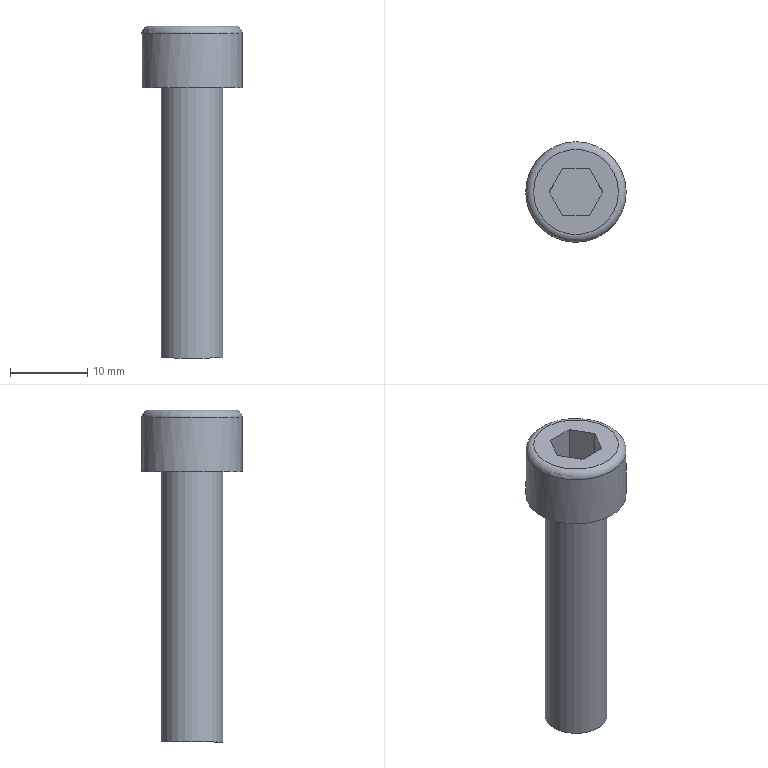Part | STEP file | Tube necking machine_id262_x_t | 1 solid | 13 faces | box 13 x 13 x 43 mm | volume 2648 mm3 | plane 10 | cylinder 2 | torus 1 | commonest cylinder face diameters 8 x1 13 x1
STEP:
#1=CARTESIAN_POINT('',(0.,0.,0.));
#2=DIRECTION('',(0.,0.,1.));
#3=DIRECTION('',(1.,0.,0.));
#4=AXIS2_PLACEMENT_3D('',#1,#2,#3);
#5=CARTESIAN_POINT('',(42.5,122.,246.));
#6=VERTEX_POINT('',#5);
#7=CARTESIAN_POINT('',(48.,122.,246.));
#8=DIRECTION('',(0.,0.,1.));
#9=DIRECTION('',(-1.,0.,0.));
#10=AXIS2_PLACEMENT_3D('',#7,#8,#9);
#11=CIRCLE('',#10,5.5);
#12=CARTESIAN_POINT('',(54.5,122.,246.));
#13=DIRECTION('',(0.,0.,-1.));
#14=DIRECTION('',(-1.,0.,0.));
#15=AXIS2_PLACEMENT_3D('',#12,#13,#14);
#16=PLANE('',#15);
#17=CARTESIAN_POINT('',(12.,0.));
#18=CARTESIAN_POINT('',(12.,-9.526));
#19=CARTESIAN_POINT('',(3.75,-4.763));
#20=CARTESIAN_POINT('',(-4.5,0.));
#21=CARTESIAN_POINT('',(3.75,4.763));
#22=CARTESIAN_POINT('',(12.,9.526));
#23=CARTESIAN_POINT('',(12.,0.));
#24=(BOUNDED_CURVE()B_SPLINE_CURVE(2,(#17,#18,#19,#20,#21,#22,#23),.UNSPECIFIED.,.T.,.F.)B_SPLINE_CURVE_WITH_KNOTS((1,2,2,2,2,1),(-2.094,0.,2.094,4.189,6.283,8.378),.UNSPECIFIED.)CURVE()GEOMETRIC_REPRESENTATION_ITEM()RATIONAL_B_SPLINE_CURVE((1.,0.5,1.,0.5,1.,0.5,1.))REPRESENTATION_ITEM(''));
#25=(GEOMETRIC_REPRESENTATION_CONTEXT(2)PARAMETRIC_REPRESENTATION_CONTEXT()REPRESENTATION_CONTEXT('',''));
#26=DEFINITIONAL_REPRESENTATION('',(#24),#25);
#27=PCURVE('',#16,#26);
#28=CARTESIAN_POINT('',(48.,122.,245.));
#29=DIRECTION('',(0.,0.,-1.));
#30=DIRECTION('',(-1.,0.,0.));
#31=AXIS2_PLACEMENT_3D('',#28,#29,#30);
#32=TOROIDAL_SURFACE('',#31,5.5,1.);
#33=CARTESIAN_POINT('',(6.283,4.712));
#34=DIRECTION('',(-1.,0.));
#35=VECTOR('',#34,1.);
#36=LINE('',#33,#35);
#37=(GEOMETRIC_REPRESENTATION_CONTEXT(2)PARAMETRIC_REPRESENTATION_CONTEXT()REPRESENTATION_CONTEXT('',''));
#38=DEFINITIONAL_REPRESENTATION('',(#36),#37);
#39=PCURVE('',#32,#38);
#40=SURFACE_CURVE('',#11,(#27,#39),.PCURVE_S1.);
#41=EDGE_CURVE('',#6,#6,#40,.T.);
#42=ORIENTED_EDGE('',*,*,#41,.T.);
#43=EDGE_LOOP('',(#42));
#44=FACE_BOUND('',#43,.T.);
#45=CARTESIAN_POINT('',(49.732,119.,246.));
#46=VERTEX_POINT('',#45);
#47=CARTESIAN_POINT('',(46.268,119.,246.));
#48=VERTEX_POINT('',#47);
#49=CARTESIAN_POINT('',(46.268,119.,246.));
#50=DIRECTION('',(-1.,0.,0.));
#51=VECTOR('',#50,1.);
#52=LINE('',#49,#51);
#53=CARTESIAN_POINT('',(8.232,-3.));
#54=DIRECTION('',(1.,0.));
#55=VECTOR('',#54,1.);
#56=LINE('',#53,#55);
#57=(GEOMETRIC_REPRESENTATION_CONTEXT(2)PARAMETRIC_REPRESENTATION_CONTEXT()REPRESENTATION_CONTEXT('',''));
#58=DEFINITIONAL_REPRESENTATION('',(#56),#57);
#59=PCURVE('',#16,#58);
#60=CARTESIAN_POINT('',(46.268,119.,240.72));
#61=DIRECTION('',(0.,1.,0.));
#62=DIRECTION('',(1.,0.,0.));
#63=AXIS2_PLACEMENT_3D('',#60,#61,#62);
#64=PLANE('',#63);
#65=CARTESIAN_POINT('',(0.,-5.28));
#66=DIRECTION('',(-1.,0.));
#67=VECTOR('',#66,1.);
#68=LINE('',#65,#67);
#69=(GEOMETRIC_REPRESENTATION_CONTEXT(2)PARAMETRIC_REPRESENTATION_CONTEXT()REPRESENTATION_CONTEXT('',''));
#70=DEFINITIONAL_REPRESENTATION('',(#68),#69);
#71=PCURVE('',#64,#70);
#72=SURFACE_CURVE('',#52,(#59,#71),.PCURVE_S1.);
#73=EDGE_CURVE('',#46,#48,#72,.T.);
#74=ORIENTED_EDGE('',*,*,#73,.T.);
#75=CARTESIAN_POINT('',(44.536,122.,246.));
#76=VERTEX_POINT('',#75);
#77=CARTESIAN_POINT('',(44.536,122.,246.));
#78=DIRECTION('',(-0.5,0.866,0.));
#79=VECTOR('',#78,1.);
#80=LINE('',#77,#79);
#81=CARTESIAN_POINT('',(9.964,0.));
#82=DIRECTION('',(0.5,0.866));
#83=VECTOR('',#82,1.);
#84=LINE('',#81,#83);
#85=(GEOMETRIC_REPRESENTATION_CONTEXT(2)PARAMETRIC_REPRESENTATION_CONTEXT()REPRESENTATION_CONTEXT('',''));
#86=DEFINITIONAL_REPRESENTATION('',(#84),#85);
#87=PCURVE('',#16,#86);
#88=CARTESIAN_POINT('',(44.536,122.,240.72));
#89=DIRECTION('',(0.866,0.5,0.));
#90=DIRECTION('',(0.5,-0.866,0.));
#91=AXIS2_PLACEMENT_3D('',#88,#89,#90);
#92=PLANE('',#91);
#93=CARTESIAN_POINT('',(0.,-5.28));
#94=DIRECTION('',(-1.,0.));
#95=VECTOR('',#94,1.);
#96=LINE('',#93,#95);
#97=(GEOMETRIC_REPRESENTATION_CONTEXT(2)PARAMETRIC_REPRESENTATION_CONTEXT()REPRESENTATION_CONTEXT('',''));
#98=DEFINITIONAL_REPRESENTATION('',(#96),#97);
#99=PCURVE('',#92,#98);
#100=SURFACE_CURVE('',#80,(#87,#99),.PCURVE_S1.);
#101=EDGE_CURVE('',#48,#76,#100,.T.);
#102=ORIENTED_EDGE('',*,*,#101,.T.);
#103=CARTESIAN_POINT('',(46.268,125.,246.));
#104=VERTEX_POINT('',#103);
#105=CARTESIAN_POINT('',(46.268,125.,246.));
#106=DIRECTION('',(0.5,0.866,0.));
#107=VECTOR('',#106,1.);
#108=LINE('',#105,#107);
#109=CARTESIAN_POINT('',(8.232,3.));
#110=DIRECTION('',(-0.5,0.866));
#111=VECTOR('',#110,1.);
#112=LINE('',#109,#111);
#113=(GEOMETRIC_REPRESENTATION_CONTEXT(2)PARAMETRIC_REPRESENTATION_CONTEXT()REPRESENTATION_CONTEXT('',''));
#114=DEFINITIONAL_REPRESENTATION('',(#112),#113);
#115=PCURVE('',#16,#114);
#116=CARTESIAN_POINT('',(46.268,125.,240.72));
#117=DIRECTION('',(0.866,-0.5,0.));
#118=DIRECTION('',(-0.5,-0.866,0.));
#119=AXIS2_PLACEMENT_3D('',#116,#117,#118);
#120=PLANE('',#119);
#121=CARTESIAN_POINT('',(0.,-5.28));
#122=DIRECTION('',(-1.,0.));
#123=VECTOR('',#122,1.);
#124=LINE('',#121,#123);
#125=(GEOMETRIC_REPRESENTATION_CONTEXT(2)PARAMETRIC_REPRESENTATION_CONTEXT()REPRESENTATION_CONTEXT('',''));
#126=DEFINITIONAL_REPRESENTATION('',(#124),#125);
#127=PCURVE('',#120,#126);
#128=SURFACE_CURVE('',#108,(#115,#127),.PCURVE_S1.);
#129=EDGE_CURVE('',#76,#104,#128,.T.);
#130=ORIENTED_EDGE('',*,*,#129,.T.);
#131=CARTESIAN_POINT('',(49.732,125.,246.));
#132=VERTEX_POINT('',#131);
#133=CARTESIAN_POINT('',(49.732,125.,246.));
#134=DIRECTION('',(1.,0.,0.));
#135=VECTOR('',#134,1.);
#136=LINE('',#133,#135);
#137=CARTESIAN_POINT('',(4.768,3.));
#138=DIRECTION('',(-1.,0.));
#139=VECTOR('',#138,1.);
#140=LINE('',#137,#139);
#141=(GEOMETRIC_REPRESENTATION_CONTEXT(2)PARAMETRIC_REPRESENTATION_CONTEXT()REPRESENTATION_CONTEXT('',''));
#142=DEFINITIONAL_REPRESENTATION('',(#140),#141);
#143=PCURVE('',#16,#142);
#144=CARTESIAN_POINT('',(49.732,125.,240.72));
#145=DIRECTION('',(0.,-1.,0.));
#146=DIRECTION('',(-1.,0.,0.));
#147=AXIS2_PLACEMENT_3D('',#144,#145,#146);
#148=PLANE('',#147);
#149=CARTESIAN_POINT('',(0.,-5.28));
#150=DIRECTION('',(-1.,0.));
#151=VECTOR('',#150,1.);
#152=LINE('',#149,#151);
#153=(GEOMETRIC_REPRESENTATION_CONTEXT(2)PARAMETRIC_REPRESENTATION_CONTEXT()REPRESENTATION_CONTEXT('',''));
#154=DEFINITIONAL_REPRESENTATION('',(#152),#153);
#155=PCURVE('',#148,#154);
#156=SURFACE_CURVE('',#136,(#143,#155),.PCURVE_S1.);
#157=EDGE_CURVE('',#104,#132,#156,.T.);
#158=ORIENTED_EDGE('',*,*,#157,.T.);
#159=CARTESIAN_POINT('',(51.464,122.,246.));
#160=VERTEX_POINT('',#159);
#161=CARTESIAN_POINT('',(51.464,122.,246.));
#162=DIRECTION('',(0.5,-0.866,0.));
#163=VECTOR('',#162,1.);
#164=LINE('',#161,#163);
#165=CARTESIAN_POINT('',(3.036,0.));
#166=DIRECTION('',(-0.5,-0.866));
#167=VECTOR('',#166,1.);
#168=LINE('',#165,#167);
#169=(GEOMETRIC_REPRESENTATION_CONTEXT(2)PARAMETRIC_REPRESENTATION_CONTEXT()REPRESENTATION_CONTEXT('',''));
#170=DEFINITIONAL_REPRESENTATION('',(#168),#169);
#171=PCURVE('',#16,#170);
#172=CARTESIAN_POINT('',(51.464,122.,240.72));
#173=DIRECTION('',(-0.866,-0.5,0.));
#174=DIRECTION('',(-0.5,0.866,0.));
#175=AXIS2_PLACEMENT_3D('',#172,#173,#174);
#176=PLANE('',#175);
#177=CARTESIAN_POINT('',(0.,-5.28));
#178=DIRECTION('',(-1.,0.));
#179=VECTOR('',#178,1.);
#180=LINE('',#177,#179);
#181=(GEOMETRIC_REPRESENTATION_CONTEXT(2)PARAMETRIC_REPRESENTATION_CONTEXT()REPRESENTATION_CONTEXT('',''));
#182=DEFINITIONAL_REPRESENTATION('',(#180),#181);
#183=PCURVE('',#176,#182);
#184=SURFACE_CURVE('',#164,(#171,#183),.PCURVE_S1.);
#185=EDGE_CURVE('',#132,#160,#184,.T.);
#186=ORIENTED_EDGE('',*,*,#185,.T.);
#187=CARTESIAN_POINT('',(49.732,119.,246.));
#188=DIRECTION('',(-0.5,-0.866,0.));
#189=VECTOR('',#188,1.);
#190=LINE('',#187,#189);
#191=CARTESIAN_POINT('',(4.768,-3.));
#192=DIRECTION('',(0.5,-0.866));
#193=VECTOR('',#192,1.);
#194=LINE('',#191,#193);
#195=(GEOMETRIC_REPRESENTATION_CONTEXT(2)PARAMETRIC_REPRESENTATION_CONTEXT()REPRESENTATION_CONTEXT('',''));
#196=DEFINITIONAL_REPRESENTATION('',(#194),#195);
#197=PCURVE('',#16,#196);
#198=CARTESIAN_POINT('',(49.732,119.,240.72));
#199=DIRECTION('',(-0.866,0.5,0.));
#200=DIRECTION('',(0.5,0.866,0.));
#201=AXIS2_PLACEMENT_3D('',#198,#199,#200);
#202=PLANE('',#201);
#203=CARTESIAN_POINT('',(0.,-5.28));
#204=DIRECTION('',(-1.,0.));
#205=VECTOR('',#204,1.);
#206=LINE('',#203,#205);
#207=(GEOMETRIC_REPRESENTATION_CONTEXT(2)PARAMETRIC_REPRESENTATION_CONTEXT()REPRESENTATION_CONTEXT('',''));
#208=DEFINITIONAL_REPRESENTATION('',(#206),#207);
#209=PCURVE('',#202,#208);
#210=SURFACE_CURVE('',#190,(#197,#209),.PCURVE_S1.);
#211=EDGE_CURVE('',#160,#46,#210,.T.);
#212=ORIENTED_EDGE('',*,*,#211,.T.);
#213=EDGE_LOOP('',(#74,#102,#130,#158,#186,#212));
#214=FACE_BOUND('',#213,.T.);
#215=ADVANCED_FACE('',(#44,#214),#16,.F.);
#216=CARTESIAN_POINT('',(41.5,122.,245.));
#217=VERTEX_POINT('',#216);
#218=CARTESIAN_POINT('',(54.5,122.,245.));
#219=VERTEX_POINT('',#218);
#220=CARTESIAN_POINT('',(48.,122.,245.));
#221=DIRECTION('',(0.,0.,-1.));
#222=DIRECTION('',(-1.,0.,0.));
#223=AXIS2_PLACEMENT_3D('',#220,#221,#222);
#224=CIRCLE('',#223,6.5);
#225=CARTESIAN_POINT('',(48.,122.,216.1));
#226=DIRECTION('',(0.,0.,1.));
#227=DIRECTION('',(1.,0.,0.));
#228=AXIS2_PLACEMENT_3D('',#225,#226,#227);
#229=CYLINDRICAL_SURFACE('',#228,6.5);
#230=CARTESIAN_POINT('',(3.142,28.9));
#231=DIRECTION('',(-1.,0.));
#232=VECTOR('',#231,1.);
#233=LINE('',#230,#232);
#234=(GEOMETRIC_REPRESENTATION_CONTEXT(2)PARAMETRIC_REPRESENTATION_CONTEXT()REPRESENTATION_CONTEXT('',''));
#235=DEFINITIONAL_REPRESENTATION('',(#233),#234);
#236=PCURVE('',#229,#235);
#237=CARTESIAN_POINT('',(0.,6.283));
#238=DIRECTION('',(1.,0.));
#239=VECTOR('',#238,1.);
#240=LINE('',#237,#239);
#241=(GEOMETRIC_REPRESENTATION_CONTEXT(2)PARAMETRIC_REPRESENTATION_CONTEXT()REPRESENTATION_CONTEXT('',''));
#242=DEFINITIONAL_REPRESENTATION('',(#240),#241);
#243=PCURVE('',#32,#242);
#244=SURFACE_CURVE('',#224,(#236,#243),.PCURVE_S1.);
#245=EDGE_CURVE('',#217,#219,#244,.T.);
#246=ORIENTED_EDGE('',*,*,#245,.T.);
#247=CARTESIAN_POINT('',(54.5,122.,238.));
#248=VERTEX_POINT('',#247);
#249=CARTESIAN_POINT('',(54.5,122.,238.));
#250=CARTESIAN_POINT('',(54.5,122.,245.));
#251=B_SPLINE_CURVE_WITH_KNOTS('',1,(#249,#250),.UNSPECIFIED.,.F.,.F.,(2,2),(21.9,28.9),.PIECEWISE_BEZIER_KNOTS.);
#252=CARTESIAN_POINT('',(0.,0.));
#253=DIRECTION('',(0.,1.));
#254=VECTOR('',#253,1.);
#255=LINE('',#252,#254);
#256=(GEOMETRIC_REPRESENTATION_CONTEXT(2)PARAMETRIC_REPRESENTATION_CONTEXT()REPRESENTATION_CONTEXT('',''));
#257=DEFINITIONAL_REPRESENTATION('',(#255),#256);
#258=PCURVE('',#229,#257);
#259=CARTESIAN_POINT('',(6.283,0.));
#260=DIRECTION('',(0.,1.));
#261=VECTOR('',#260,1.);
#262=LINE('',#259,#261);
#263=(GEOMETRIC_REPRESENTATION_CONTEXT(2)PARAMETRIC_REPRESENTATION_CONTEXT()REPRESENTATION_CONTEXT('',''));
#264=DEFINITIONAL_REPRESENTATION('',(#262),#263);
#265=PCURVE('',#229,#264);
#266=SEAM_CURVE('',#251,(#258,#265),.PCURVE_S1.);
#267=EDGE_CURVE('',#248,#219,#266,.T.);
#268=ORIENTED_EDGE('',*,*,#267,.F.);
#269=CARTESIAN_POINT('',(48.,122.,238.));
#270=DIRECTION('',(0.,0.,1.));
#271=DIRECTION('',(1.,0.,0.));
#272=AXIS2_PLACEMENT_3D('',#269,#270,#271);
#273=CIRCLE('',#272,6.5);
#274=CARTESIAN_POINT('',(0.,21.9));
#275=DIRECTION('',(1.,0.));
#276=VECTOR('',#275,1.);
#277=LINE('',#274,#276);
#278=(GEOMETRIC_REPRESENTATION_CONTEXT(2)PARAMETRIC_REPRESENTATION_CONTEXT()REPRESENTATION_CONTEXT('',''));
#279=DEFINITIONAL_REPRESENTATION('',(#277),#278);
#280=PCURVE('',#229,#279);
#281=CARTESIAN_POINT('',(52.,122.,238.));
#282=DIRECTION('',(0.,0.,1.));
#283=DIRECTION('',(1.,0.,0.));
#284=AXIS2_PLACEMENT_3D('',#281,#282,#283);
#285=PLANE('',#284);
#286=CARTESIAN_POINT('',(-4.,0.));
#287=DIRECTION('',(1.,0.));
#288=AXIS2_PLACEMENT_2D('',#286,#287);
#289=CIRCLE('',#288,6.5);
#290=(GEOMETRIC_REPRESENTATION_CONTEXT(2)PARAMETRIC_REPRESENTATION_CONTEXT()REPRESENTATION_CONTEXT('',''));
#291=DEFINITIONAL_REPRESENTATION('',(#289),#290);
#292=PCURVE('',#285,#291);
#293=SURFACE_CURVE('',#273,(#280,#292),.PCURVE_S1.);
#294=EDGE_CURVE('',#248,#248,#293,.T.);
#295=ORIENTED_EDGE('',*,*,#294,.T.);
#296=ORIENTED_EDGE('',*,*,#267,.T.);
#297=CARTESIAN_POINT('',(48.,122.,245.));
#298=DIRECTION('',(0.,0.,-1.));
#299=DIRECTION('',(-1.,0.,0.));
#300=AXIS2_PLACEMENT_3D('',#297,#298,#299);
#301=CIRCLE('',#300,6.5);
#302=CARTESIAN_POINT('',(9.425,28.9));
#303=DIRECTION('',(-1.,0.));
#304=VECTOR('',#303,1.);
#305=LINE('',#302,#304);
#306=(GEOMETRIC_REPRESENTATION_CONTEXT(2)PARAMETRIC_REPRESENTATION_CONTEXT()REPRESENTATION_CONTEXT('',''));
#307=DEFINITIONAL_REPRESENTATION('',(#305),#306);
#308=PCURVE('',#229,#307);
#309=CARTESIAN_POINT('',(0.,6.283));
#310=DIRECTION('',(1.,0.));
#311=VECTOR('',#310,1.);
#312=LINE('',#309,#311);
#313=(GEOMETRIC_REPRESENTATION_CONTEXT(2)PARAMETRIC_REPRESENTATION_CONTEXT()REPRESENTATION_CONTEXT('',''));
#314=DEFINITIONAL_REPRESENTATION('',(#312),#313);
#315=PCURVE('',#32,#314);
#316=SURFACE_CURVE('',#301,(#308,#315),.PCURVE_S1.);
#317=EDGE_CURVE('',#219,#217,#316,.T.);
#318=ORIENTED_EDGE('',*,*,#317,.T.);
#319=EDGE_LOOP('',(#246,#268,#295,#296,#318));
#320=FACE_BOUND('',#319,.T.);
#321=ADVANCED_FACE('',(#320),#229,.T.);
#322=ORIENTED_EDGE('',*,*,#294,.F.);
#323=EDGE_LOOP('',(#322));
#324=FACE_BOUND('',#323,.T.);
#325=CARTESIAN_POINT('',(52.,122.,238.));
#326=VERTEX_POINT('',#325);
#327=CARTESIAN_POINT('',(48.,122.,238.));
#328=DIRECTION('',(0.,0.,1.));
#329=DIRECTION('',(1.,0.,0.));
#330=AXIS2_PLACEMENT_3D('',#327,#328,#329);
#331=CIRCLE('',#330,4.);
#332=CARTESIAN_POINT('',(-4.,0.));
#333=DIRECTION('',(1.,0.));
#334=AXIS2_PLACEMENT_2D('',#332,#333);
#335=CIRCLE('',#334,4.);
#336=(GEOMETRIC_REPRESENTATION_CONTEXT(2)PARAMETRIC_REPRESENTATION_CONTEXT()REPRESENTATION_CONTEXT('',''));
#337=DEFINITIONAL_REPRESENTATION('',(#335),#336);
#338=PCURVE('',#285,#337);
#339=CARTESIAN_POINT('',(48.,122.,216.1));
#340=DIRECTION('',(0.,0.,1.));
#341=DIRECTION('',(1.,0.,0.));
#342=AXIS2_PLACEMENT_3D('',#339,#340,#341);
#343=CYLINDRICAL_SURFACE('',#342,4.);
#344=CARTESIAN_POINT('',(0.,21.9));
#345=DIRECTION('',(1.,0.));
#346=VECTOR('',#345,1.);
#347=LINE('',#344,#346);
#348=(GEOMETRIC_REPRESENTATION_CONTEXT(2)PARAMETRIC_REPRESENTATION_CONTEXT()REPRESENTATION_CONTEXT('',''));
#349=DEFINITIONAL_REPRESENTATION('',(#347),#348);
#350=PCURVE('',#343,#349);
#351=SURFACE_CURVE('',#331,(#338,#350),.PCURVE_S1.);
#352=EDGE_CURVE('',#326,#326,#351,.T.);
#353=ORIENTED_EDGE('',*,*,#352,.T.);
#354=EDGE_LOOP('',(#353));
#355=FACE_BOUND('',#354,.T.);
#356=ADVANCED_FACE('',(#324,#355),#285,.F.);
#357=ORIENTED_EDGE('',*,*,#352,.F.);
#358=CARTESIAN_POINT('',(52.,122.,203.));
#359=VERTEX_POINT('',#358);
#360=CARTESIAN_POINT('',(52.,122.,203.));
#361=CARTESIAN_POINT('',(52.,122.,238.));
#362=B_SPLINE_CURVE_WITH_KNOTS('',1,(#360,#361),.UNSPECIFIED.,.F.,.F.,(2,2),(-13.1,21.9),.PIECEWISE_BEZIER_KNOTS.);
#363=CARTESIAN_POINT('',(0.,0.));
#364=DIRECTION('',(0.,1.));
#365=VECTOR('',#364,1.);
#366=LINE('',#363,#365);
#367=(GEOMETRIC_REPRESENTATION_CONTEXT(2)PARAMETRIC_REPRESENTATION_CONTEXT()REPRESENTATION_CONTEXT('',''));
#368=DEFINITIONAL_REPRESENTATION('',(#366),#367);
#369=PCURVE('',#343,#368);
#370=CARTESIAN_POINT('',(6.283,0.));
#371=DIRECTION('',(0.,1.));
#372=VECTOR('',#371,1.);
#373=LINE('',#370,#372);
#374=(GEOMETRIC_REPRESENTATION_CONTEXT(2)PARAMETRIC_REPRESENTATION_CONTEXT()REPRESENTATION_CONTEXT('',''));
#375=DEFINITIONAL_REPRESENTATION('',(#373),#374);
#376=PCURVE('',#343,#375);
#377=SEAM_CURVE('',#362,(#369,#376),.PCURVE_S1.);
#378=EDGE_CURVE('',#359,#326,#377,.T.);
#379=ORIENTED_EDGE('',*,*,#378,.F.);
#380=CARTESIAN_POINT('',(48.,122.,203.));
#381=DIRECTION('',(0.,0.,1.));
#382=DIRECTION('',(1.,0.,0.));
#383=AXIS2_PLACEMENT_3D('',#380,#381,#382);
#384=CIRCLE('',#383,4.);
#385=CARTESIAN_POINT('',(0.,-13.1));
#386=DIRECTION('',(1.,0.));
#387=VECTOR('',#386,1.);
#388=LINE('',#385,#387);
#389=(GEOMETRIC_REPRESENTATION_CONTEXT(2)PARAMETRIC_REPRESENTATION_CONTEXT()REPRESENTATION_CONTEXT('',''));
#390=DEFINITIONAL_REPRESENTATION('',(#388),#389);
#391=PCURVE('',#343,#390);
#392=CARTESIAN_POINT('',(48.,122.,203.));
#393=DIRECTION('',(0.,0.,1.));
#394=DIRECTION('',(1.,0.,0.));
#395=AXIS2_PLACEMENT_3D('',#392,#393,#394);
#396=PLANE('',#395);
#397=CARTESIAN_POINT('',(0.,0.));
#398=DIRECTION('',(1.,0.));
#399=AXIS2_PLACEMENT_2D('',#397,#398);
#400=CIRCLE('',#399,4.);
#401=(GEOMETRIC_REPRESENTATION_CONTEXT(2)PARAMETRIC_REPRESENTATION_CONTEXT()REPRESENTATION_CONTEXT('',''));
#402=DEFINITIONAL_REPRESENTATION('',(#400),#401);
#403=PCURVE('',#396,#402);
#404=SURFACE_CURVE('',#384,(#391,#403),.PCURVE_S1.);
#405=EDGE_CURVE('',#359,#359,#404,.T.);
#406=ORIENTED_EDGE('',*,*,#405,.T.);
#407=ORIENTED_EDGE('',*,*,#378,.T.);
#408=EDGE_LOOP('',(#357,#379,#406,#407));
#409=FACE_BOUND('',#408,.T.);
#410=ADVANCED_FACE('',(#409),#343,.T.);
#411=ORIENTED_EDGE('',*,*,#405,.F.);
#412=EDGE_LOOP('',(#411));
#413=FACE_BOUND('',#412,.T.);
#414=ADVANCED_FACE('',(#413),#396,.F.);
#415=ORIENTED_EDGE('',*,*,#73,.F.);
#416=CARTESIAN_POINT('',(49.732,119.,240.72));
#417=VERTEX_POINT('',#416);
#418=CARTESIAN_POINT('',(49.732,119.,240.72));
#419=DIRECTION('',(0.,0.,1.));
#420=VECTOR('',#419,1.);
#421=LINE('',#418,#420);
#422=CARTESIAN_POINT('',(3.464,0.));
#423=DIRECTION('',(0.,-1.));
#424=VECTOR('',#423,1.);
#425=LINE('',#422,#424);
#426=(GEOMETRIC_REPRESENTATION_CONTEXT(2)PARAMETRIC_REPRESENTATION_CONTEXT()REPRESENTATION_CONTEXT('',''));
#427=DEFINITIONAL_REPRESENTATION('',(#425),#426);
#428=PCURVE('',#64,#427);
#429=CARTESIAN_POINT('',(0.,0.));
#430=DIRECTION('',(0.,-1.));
#431=VECTOR('',#430,1.);
#432=LINE('',#429,#431);
#433=(GEOMETRIC_REPRESENTATION_CONTEXT(2)PARAMETRIC_REPRESENTATION_CONTEXT()REPRESENTATION_CONTEXT('',''));
#434=DEFINITIONAL_REPRESENTATION('',(#432),#433);
#435=PCURVE('',#202,#434);
#436=SURFACE_CURVE('',#421,(#428,#435),.PCURVE_S1.);
#437=EDGE_CURVE('',#417,#46,#436,.T.);
#438=ORIENTED_EDGE('',*,*,#437,.F.);
#439=CARTESIAN_POINT('',(46.268,119.,240.72));
#440=VERTEX_POINT('',#439);
#441=CARTESIAN_POINT('',(46.268,119.,240.72));
#442=DIRECTION('',(1.,0.,0.));
#443=VECTOR('',#442,1.);
#444=LINE('',#441,#443);
#445=CARTESIAN_POINT('',(0.,0.));
#446=DIRECTION('',(1.,0.));
#447=VECTOR('',#446,1.);
#448=LINE('',#445,#447);
#449=(GEOMETRIC_REPRESENTATION_CONTEXT(2)PARAMETRIC_REPRESENTATION_CONTEXT()REPRESENTATION_CONTEXT('',''));
#450=DEFINITIONAL_REPRESENTATION('',(#448),#449);
#451=PCURVE('',#64,#450);
#452=CARTESIAN_POINT('',(48.,122.,240.72));
#453=DIRECTION('',(0.,0.,-1.));
#454=DIRECTION('',(-1.,0.,0.));
#455=AXIS2_PLACEMENT_3D('',#452,#453,#454);
#456=PLANE('',#455);
#457=CARTESIAN_POINT('',(1.732,-3.));
#458=DIRECTION('',(-1.,0.));
#459=VECTOR('',#458,1.);
#460=LINE('',#457,#459);
#461=(GEOMETRIC_REPRESENTATION_CONTEXT(2)PARAMETRIC_REPRESENTATION_CONTEXT()REPRESENTATION_CONTEXT('',''));
#462=DEFINITIONAL_REPRESENTATION('',(#460),#461);
#463=PCURVE('',#456,#462);
#464=SURFACE_CURVE('',#444,(#451,#463),.PCURVE_S1.);
#465=EDGE_CURVE('',#440,#417,#464,.T.);
#466=ORIENTED_EDGE('',*,*,#465,.F.);
#467=CARTESIAN_POINT('',(46.268,119.,240.72));
#468=DIRECTION('',(0.,0.,1.));
#469=VECTOR('',#468,1.);
#470=LINE('',#467,#469);
#471=CARTESIAN_POINT('',(0.,0.));
#472=DIRECTION('',(0.,-1.));
#473=VECTOR('',#472,1.);
#474=LINE('',#471,#473);
#475=(GEOMETRIC_REPRESENTATION_CONTEXT(2)PARAMETRIC_REPRESENTATION_CONTEXT()REPRESENTATION_CONTEXT('',''));
#476=DEFINITIONAL_REPRESENTATION('',(#474),#475);
#477=PCURVE('',#64,#476);
#478=CARTESIAN_POINT('',(3.464,0.));
#479=DIRECTION('',(0.,-1.));
#480=VECTOR('',#479,1.);
#481=LINE('',#478,#480);
#482=(GEOMETRIC_REPRESENTATION_CONTEXT(2)PARAMETRIC_REPRESENTATION_CONTEXT()REPRESENTATION_CONTEXT('',''));
#483=DEFINITIONAL_REPRESENTATION('',(#481),#482);
#484=PCURVE('',#92,#483);
#485=SURFACE_CURVE('',#470,(#477,#484),.PCURVE_S1.);
#486=EDGE_CURVE('',#440,#48,#485,.T.);
#487=ORIENTED_EDGE('',*,*,#486,.T.);
#488=EDGE_LOOP('',(#415,#438,#466,#487));
#489=FACE_BOUND('',#488,.T.);
#490=ADVANCED_FACE('',(#489),#64,.T.);
#491=ORIENTED_EDGE('',*,*,#211,.F.);
#492=CARTESIAN_POINT('',(51.464,122.,240.72));
#493=VERTEX_POINT('',#492);
#494=CARTESIAN_POINT('',(51.464,122.,240.72));
#495=DIRECTION('',(0.,0.,1.));
#496=VECTOR('',#495,1.);
#497=LINE('',#494,#496);
#498=CARTESIAN_POINT('',(3.464,0.));
#499=DIRECTION('',(0.,-1.));
#500=VECTOR('',#499,1.);
#501=LINE('',#498,#500);
#502=(GEOMETRIC_REPRESENTATION_CONTEXT(2)PARAMETRIC_REPRESENTATION_CONTEXT()REPRESENTATION_CONTEXT('',''));
#503=DEFINITIONAL_REPRESENTATION('',(#501),#502);
#504=PCURVE('',#202,#503);
#505=CARTESIAN_POINT('',(0.,0.));
#506=DIRECTION('',(0.,-1.));
#507=VECTOR('',#506,1.);
#508=LINE('',#505,#507);
#509=(GEOMETRIC_REPRESENTATION_CONTEXT(2)PARAMETRIC_REPRESENTATION_CONTEXT()REPRESENTATION_CONTEXT('',''));
#510=DEFINITIONAL_REPRESENTATION('',(#508),#509);
#511=PCURVE('',#176,#510);
#512=SURFACE_CURVE('',#497,(#504,#511),.PCURVE_S1.);
#513=EDGE_CURVE('',#493,#160,#512,.T.);
#514=ORIENTED_EDGE('',*,*,#513,.F.);
#515=CARTESIAN_POINT('',(49.732,119.,240.72));
#516=DIRECTION('',(0.5,0.866,0.));
#517=VECTOR('',#516,1.);
#518=LINE('',#515,#517);
#519=CARTESIAN_POINT('',(0.,0.));
#520=DIRECTION('',(1.,0.));
#521=VECTOR('',#520,1.);
#522=LINE('',#519,#521);
#523=(GEOMETRIC_REPRESENTATION_CONTEXT(2)PARAMETRIC_REPRESENTATION_CONTEXT()REPRESENTATION_CONTEXT('',''));
#524=DEFINITIONAL_REPRESENTATION('',(#522),#523);
#525=PCURVE('',#202,#524);
#526=CARTESIAN_POINT('',(-1.732,-3.));
#527=DIRECTION('',(-0.5,0.866));
#528=VECTOR('',#527,1.);
#529=LINE('',#526,#528);
#530=(GEOMETRIC_REPRESENTATION_CONTEXT(2)PARAMETRIC_REPRESENTATION_CONTEXT()REPRESENTATION_CONTEXT('',''));
#531=DEFINITIONAL_REPRESENTATION('',(#529),#530);
#532=PCURVE('',#456,#531);
#533=SURFACE_CURVE('',#518,(#525,#532),.PCURVE_S1.);
#534=EDGE_CURVE('',#417,#493,#533,.T.);
#535=ORIENTED_EDGE('',*,*,#534,.F.);
#536=ORIENTED_EDGE('',*,*,#437,.T.);
#537=EDGE_LOOP('',(#491,#514,#535,#536));
#538=FACE_BOUND('',#537,.T.);
#539=ADVANCED_FACE('',(#538),#202,.T.);
#540=ORIENTED_EDGE('',*,*,#185,.F.);
#541=CARTESIAN_POINT('',(49.732,125.,240.72));
#542=VERTEX_POINT('',#541);
#543=CARTESIAN_POINT('',(49.732,125.,240.72));
#544=DIRECTION('',(0.,0.,1.));
#545=VECTOR('',#544,1.);
#546=LINE('',#543,#545);
#547=CARTESIAN_POINT('',(3.464,0.));
#548=DIRECTION('',(0.,-1.));
#549=VECTOR('',#548,1.);
#550=LINE('',#547,#549);
#551=(GEOMETRIC_REPRESENTATION_CONTEXT(2)PARAMETRIC_REPRESENTATION_CONTEXT()REPRESENTATION_CONTEXT('',''));
#552=DEFINITIONAL_REPRESENTATION('',(#550),#551);
#553=PCURVE('',#176,#552);
#554=CARTESIAN_POINT('',(0.,0.));
#555=DIRECTION('',(0.,-1.));
#556=VECTOR('',#555,1.);
#557=LINE('',#554,#556);
#558=(GEOMETRIC_REPRESENTATION_CONTEXT(2)PARAMETRIC_REPRESENTATION_CONTEXT()REPRESENTATION_CONTEXT('',''));
#559=DEFINITIONAL_REPRESENTATION('',(#557),#558);
#560=PCURVE('',#148,#559);
#561=SURFACE_CURVE('',#546,(#553,#560),.PCURVE_S1.);
#562=EDGE_CURVE('',#542,#132,#561,.T.);
#563=ORIENTED_EDGE('',*,*,#562,.F.);
#564=CARTESIAN_POINT('',(51.464,122.,240.72));
#565=DIRECTION('',(-0.5,0.866,0.));
#566=VECTOR('',#565,1.);
#567=LINE('',#564,#566);
#568=CARTESIAN_POINT('',(0.,0.));
#569=DIRECTION('',(1.,0.));
#570=VECTOR('',#569,1.);
#571=LINE('',#568,#570);
#572=(GEOMETRIC_REPRESENTATION_CONTEXT(2)PARAMETRIC_REPRESENTATION_CONTEXT()REPRESENTATION_CONTEXT('',''));
#573=DEFINITIONAL_REPRESENTATION('',(#571),#572);
#574=PCURVE('',#176,#573);
#575=CARTESIAN_POINT('',(-3.464,0.));
#576=DIRECTION('',(0.5,0.866));
#577=VECTOR('',#576,1.);
#578=LINE('',#575,#577);
#579=(GEOMETRIC_REPRESENTATION_CONTEXT(2)PARAMETRIC_REPRESENTATION_CONTEXT()REPRESENTATION_CONTEXT('',''));
#580=DEFINITIONAL_REPRESENTATION('',(#578),#579);
#581=PCURVE('',#456,#580);
#582=SURFACE_CURVE('',#567,(#574,#581),.PCURVE_S1.);
#583=EDGE_CURVE('',#493,#542,#582,.T.);
#584=ORIENTED_EDGE('',*,*,#583,.F.);
#585=ORIENTED_EDGE('',*,*,#513,.T.);
#586=EDGE_LOOP('',(#540,#563,#584,#585));
#587=FACE_BOUND('',#586,.T.);
#588=ADVANCED_FACE('',(#587),#176,.T.);
#589=ORIENTED_EDGE('',*,*,#157,.F.);
#590=CARTESIAN_POINT('',(46.268,125.,240.72));
#591=VERTEX_POINT('',#590);
#592=CARTESIAN_POINT('',(46.268,125.,240.72));
#593=DIRECTION('',(0.,0.,1.));
#594=VECTOR('',#593,1.);
#595=LINE('',#592,#594);
#596=CARTESIAN_POINT('',(3.464,0.));
#597=DIRECTION('',(0.,-1.));
#598=VECTOR('',#597,1.);
#599=LINE('',#596,#598);
#600=(GEOMETRIC_REPRESENTATION_CONTEXT(2)PARAMETRIC_REPRESENTATION_CONTEXT()REPRESENTATION_CONTEXT('',''));
#601=DEFINITIONAL_REPRESENTATION('',(#599),#600);
#602=PCURVE('',#148,#601);
#603=CARTESIAN_POINT('',(0.,0.));
#604=DIRECTION('',(0.,-1.));
#605=VECTOR('',#604,1.);
#606=LINE('',#603,#605);
#607=(GEOMETRIC_REPRESENTATION_CONTEXT(2)PARAMETRIC_REPRESENTATION_CONTEXT()REPRESENTATION_CONTEXT('',''));
#608=DEFINITIONAL_REPRESENTATION('',(#606),#607);
#609=PCURVE('',#120,#608);
#610=SURFACE_CURVE('',#595,(#602,#609),.PCURVE_S1.);
#611=EDGE_CURVE('',#591,#104,#610,.T.);
#612=ORIENTED_EDGE('',*,*,#611,.F.);
#613=CARTESIAN_POINT('',(49.732,125.,240.72));
#614=DIRECTION('',(-1.,0.,0.));
#615=VECTOR('',#614,1.);
#616=LINE('',#613,#615);
#617=CARTESIAN_POINT('',(0.,0.));
#618=DIRECTION('',(1.,0.));
#619=VECTOR('',#618,1.);
#620=LINE('',#617,#619);
#621=(GEOMETRIC_REPRESENTATION_CONTEXT(2)PARAMETRIC_REPRESENTATION_CONTEXT()REPRESENTATION_CONTEXT('',''));
#622=DEFINITIONAL_REPRESENTATION('',(#620),#621);
#623=PCURVE('',#148,#622);
#624=CARTESIAN_POINT('',(-1.732,3.));
#625=DIRECTION('',(1.,0.));
#626=VECTOR('',#625,1.);
#627=LINE('',#624,#626);
#628=(GEOMETRIC_REPRESENTATION_CONTEXT(2)PARAMETRIC_REPRESENTATION_CONTEXT()REPRESENTATION_CONTEXT('',''));
#629=DEFINITIONAL_REPRESENTATION('',(#627),#628);
#630=PCURVE('',#456,#629);
#631=SURFACE_CURVE('',#616,(#623,#630),.PCURVE_S1.);
#632=EDGE_CURVE('',#542,#591,#631,.T.);
#633=ORIENTED_EDGE('',*,*,#632,.F.);
#634=ORIENTED_EDGE('',*,*,#562,.T.);
#635=EDGE_LOOP('',(#589,#612,#633,#634));
#636=FACE_BOUND('',#635,.T.);
#637=ADVANCED_FACE('',(#636),#148,.T.);
#638=ORIENTED_EDGE('',*,*,#129,.F.);
#639=CARTESIAN_POINT('',(44.536,122.,240.72));
#640=VERTEX_POINT('',#639);
#641=CARTESIAN_POINT('',(44.536,122.,240.72));
#642=DIRECTION('',(0.,0.,1.));
#643=VECTOR('',#642,1.);
#644=LINE('',#641,#643);
#645=CARTESIAN_POINT('',(3.464,0.));
#646=DIRECTION('',(0.,-1.));
#647=VECTOR('',#646,1.);
#648=LINE('',#645,#647);
#649=(GEOMETRIC_REPRESENTATION_CONTEXT(2)PARAMETRIC_REPRESENTATION_CONTEXT()REPRESENTATION_CONTEXT('',''));
#650=DEFINITIONAL_REPRESENTATION('',(#648),#649);
#651=PCURVE('',#120,#650);
#652=CARTESIAN_POINT('',(0.,0.));
#653=DIRECTION('',(0.,-1.));
#654=VECTOR('',#653,1.);
#655=LINE('',#652,#654);
#656=(GEOMETRIC_REPRESENTATION_CONTEXT(2)PARAMETRIC_REPRESENTATION_CONTEXT()REPRESENTATION_CONTEXT('',''));
#657=DEFINITIONAL_REPRESENTATION('',(#655),#656);
#658=PCURVE('',#92,#657);
#659=SURFACE_CURVE('',#644,(#651,#658),.PCURVE_S1.);
#660=EDGE_CURVE('',#640,#76,#659,.T.);
#661=ORIENTED_EDGE('',*,*,#660,.F.);
#662=CARTESIAN_POINT('',(46.268,125.,240.72));
#663=DIRECTION('',(-0.5,-0.866,0.));
#664=VECTOR('',#663,1.);
#665=LINE('',#662,#664);
#666=CARTESIAN_POINT('',(0.,0.));
#667=DIRECTION('',(1.,0.));
#668=VECTOR('',#667,1.);
#669=LINE('',#666,#668);
#670=(GEOMETRIC_REPRESENTATION_CONTEXT(2)PARAMETRIC_REPRESENTATION_CONTEXT()REPRESENTATION_CONTEXT('',''));
#671=DEFINITIONAL_REPRESENTATION('',(#669),#670);
#672=PCURVE('',#120,#671);
#673=CARTESIAN_POINT('',(1.732,3.));
#674=DIRECTION('',(0.5,-0.866));
#675=VECTOR('',#674,1.);
#676=LINE('',#673,#675);
#677=(GEOMETRIC_REPRESENTATION_CONTEXT(2)PARAMETRIC_REPRESENTATION_CONTEXT()REPRESENTATION_CONTEXT('',''));
#678=DEFINITIONAL_REPRESENTATION('',(#676),#677);
#679=PCURVE('',#456,#678);
#680=SURFACE_CURVE('',#665,(#672,#679),.PCURVE_S1.);
#681=EDGE_CURVE('',#591,#640,#680,.T.);
#682=ORIENTED_EDGE('',*,*,#681,.F.);
#683=ORIENTED_EDGE('',*,*,#611,.T.);
#684=EDGE_LOOP('',(#638,#661,#682,#683));
#685=FACE_BOUND('',#684,.T.);
#686=ADVANCED_FACE('',(#685),#120,.T.);
#687=ORIENTED_EDGE('',*,*,#101,.F.);
#688=ORIENTED_EDGE('',*,*,#486,.F.);
#689=CARTESIAN_POINT('',(44.536,122.,240.72));
#690=DIRECTION('',(0.5,-0.866,0.));
#691=VECTOR('',#690,1.);
#692=LINE('',#689,#691);
#693=CARTESIAN_POINT('',(0.,0.));
#694=DIRECTION('',(1.,0.));
#695=VECTOR('',#694,1.);
#696=LINE('',#693,#695);
#697=(GEOMETRIC_REPRESENTATION_CONTEXT(2)PARAMETRIC_REPRESENTATION_CONTEXT()REPRESENTATION_CONTEXT('',''));
#698=DEFINITIONAL_REPRESENTATION('',(#696),#697);
#699=PCURVE('',#92,#698);
#700=CARTESIAN_POINT('',(3.464,0.));
#701=DIRECTION('',(-0.5,-0.866));
#702=VECTOR('',#701,1.);
#703=LINE('',#700,#702);
#704=(GEOMETRIC_REPRESENTATION_CONTEXT(2)PARAMETRIC_REPRESENTATION_CONTEXT()REPRESENTATION_CONTEXT('',''));
#705=DEFINITIONAL_REPRESENTATION('',(#703),#704);
#706=PCURVE('',#456,#705);
#707=SURFACE_CURVE('',#692,(#699,#706),.PCURVE_S1.);
#708=EDGE_CURVE('',#640,#440,#707,.T.);
#709=ORIENTED_EDGE('',*,*,#708,.F.);
#710=ORIENTED_EDGE('',*,*,#660,.T.);
#711=EDGE_LOOP('',(#687,#688,#709,#710));
#712=FACE_BOUND('',#711,.T.);
#713=ADVANCED_FACE('',(#712),#92,.T.);
#714=ORIENTED_EDGE('',*,*,#465,.T.);
#715=ORIENTED_EDGE('',*,*,#534,.T.);
#716=ORIENTED_EDGE('',*,*,#583,.T.);
#717=ORIENTED_EDGE('',*,*,#632,.T.);
#718=ORIENTED_EDGE('',*,*,#681,.T.);
#719=ORIENTED_EDGE('',*,*,#708,.T.);
#720=EDGE_LOOP('',(#714,#715,#716,#717,#718,#719));
#721=FACE_BOUND('',#720,.T.);
#722=ADVANCED_FACE('',(#721),#456,.F.);
#723=ORIENTED_EDGE('',*,*,#245,.F.);
#724=CARTESIAN_POINT('',(42.5,122.,246.));
#725=CARTESIAN_POINT('',(42.233,122.,246.));
#726=CARTESIAN_POINT('',(41.972,122.,245.915));
#727=CARTESIAN_POINT('',(41.748,122.,245.752));
#728=CARTESIAN_POINT('',(41.585,122.,245.528));
#729=CARTESIAN_POINT('',(41.5,122.,245.267));
#730=CARTESIAN_POINT('',(41.5,122.,245.));
#731=(BOUNDED_CURVE()B_SPLINE_CURVE(6,(#724,#725,#726,#727,#728,#729,#730),.UNSPECIFIED.,.F.,.F.)B_SPLINE_CURVE_WITH_KNOTS((7,7),(-1.571,0.),.PIECEWISE_BEZIER_KNOTS.)CURVE()GEOMETRIC_REPRESENTATION_ITEM()RATIONAL_B_SPLINE_CURVE((1.031,1.01,0.9979,0.994,0.9979,1.01,1.031))REPRESENTATION_ITEM(''));
#732=CARTESIAN_POINT('',(0.,6.283));
#733=DIRECTION('',(0.,1.));
#734=VECTOR('',#733,1.);
#735=LINE('',#732,#734);
#736=(GEOMETRIC_REPRESENTATION_CONTEXT(2)PARAMETRIC_REPRESENTATION_CONTEXT()REPRESENTATION_CONTEXT('',''));
#737=DEFINITIONAL_REPRESENTATION('',(#735),#736);
#738=PCURVE('',#32,#737);
#739=CARTESIAN_POINT('',(6.283,6.283));
#740=DIRECTION('',(0.,1.));
#741=VECTOR('',#740,1.);
#742=LINE('',#739,#741);
#743=(GEOMETRIC_REPRESENTATION_CONTEXT(2)PARAMETRIC_REPRESENTATION_CONTEXT()REPRESENTATION_CONTEXT('',''));
#744=DEFINITIONAL_REPRESENTATION('',(#742),#743);
#745=PCURVE('',#32,#744);
#746=SEAM_CURVE('',#731,(#738,#745),.PCURVE_S1.);
#747=EDGE_CURVE('',#6,#217,#746,.T.);
#748=ORIENTED_EDGE('',*,*,#747,.F.);
#749=ORIENTED_EDGE('',*,*,#41,.F.);
#750=ORIENTED_EDGE('',*,*,#747,.T.);
#751=ORIENTED_EDGE('',*,*,#317,.F.);
#752=EDGE_LOOP('',(#723,#748,#749,#750,#751));
#753=FACE_BOUND('',#752,.T.);
#754=ADVANCED_FACE('',(#753),#32,.T.);
#755=CLOSED_SHELL('',(#215,#321,#356,#410,#414,#490,#539,#588,#637,#686,#713,#722,#754));
#756=MANIFOLD_SOLID_BREP('',#755);
#757=(LENGTH_UNIT()NAMED_UNIT(*)SI_UNIT(.MILLI.,.METRE.));
#758=UNCERTAINTY_MEASURE_WITH_UNIT(LENGTH_MEASURE(0.000002),#757,'','');
#759=(NAMED_UNIT(*)PLANE_ANGLE_UNIT()SI_UNIT($,.RADIAN.));
#760=(NAMED_UNIT(*)SI_UNIT($,.STERADIAN.)SOLID_ANGLE_UNIT());
#761=(GEOMETRIC_REPRESENTATION_CONTEXT(3)GLOBAL_UNCERTAINTY_ASSIGNED_CONTEXT((#758))GLOBAL_UNIT_ASSIGNED_CONTEXT((#757,#759,#760))REPRESENTATION_CONTEXT('',''));
#762=ADVANCED_BREP_SHAPE_REPRESENTATION('',(#4,#756),#761);